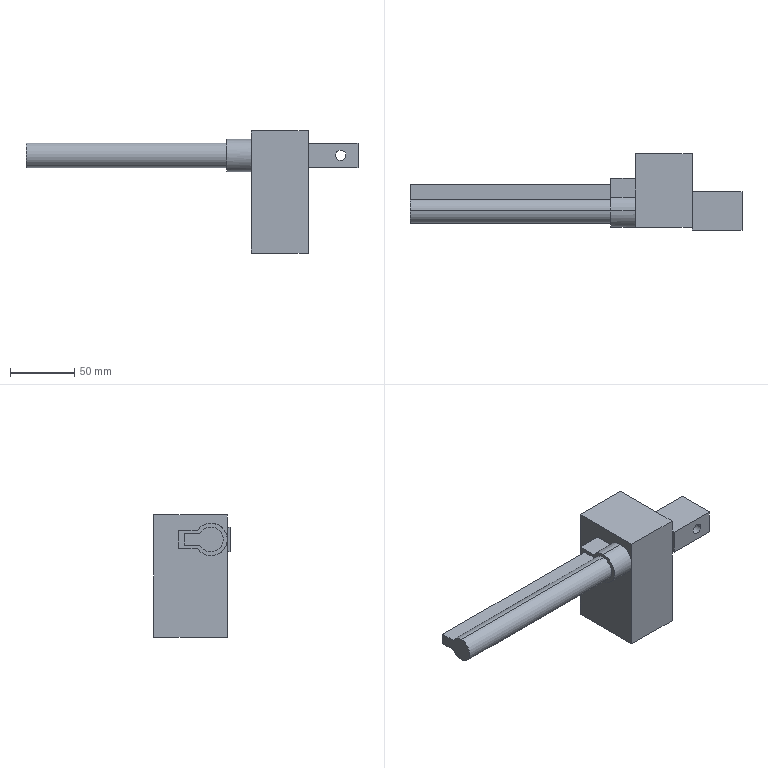Part | NX | features BREP 1 | 1 solid | 28 faces | box 259.112 x 59.436 x 95.25 mm | volume 337002 mm3 | plane 20 | cylinder 8 | commonest cylinder face diameters 19.304 x3 25.4 x3 8.255 x2
STEP:
#1=CARTESIAN_POINT('',(-19.05,25.4,6.985));
#2=VERTEX_POINT('',#1);
#3=CARTESIAN_POINT('',(-19.05,25.4,-6.985));
#4=VERTEX_POINT('',#3);
#5=CARTESIAN_POINT('',(-19.05,25.4,6.985));
#6=DIRECTION('',(0.,0.,-1.));
#7=VECTOR('',#6,1000.);
#8=LINE('',#5,#7);
#9=EDGE_CURVE('',#2,#4,#8,.T.);
#10=ORIENTED_EDGE('',*,*,#9,.T.);
#11=CARTESIAN_POINT('',(-19.05,10.607,-6.985));
#12=VERTEX_POINT('',#11);
#13=CARTESIAN_POINT('',(-19.05,25.4,-6.985));
#14=DIRECTION('',(0.,-1.,0.));
#15=VECTOR('',#14,1000.);
#16=LINE('',#13,#15);
#17=EDGE_CURVE('',#4,#12,#16,.T.);
#18=ORIENTED_EDGE('',*,*,#17,.T.);
#19=CARTESIAN_POINT('',(-19.05,0.,-12.7));
#20=VERTEX_POINT('',#19);
#21=CARTESIAN_POINT('',(-19.05,0.,0.));
#22=DIRECTION('',(-1.,0.,0.));
#23=DIRECTION('',(0.,0.8352,-0.55));
#24=AXIS2_PLACEMENT_3D('',#21,#22,#23);
#25=CIRCLE('',#24,12.7);
#26=EDGE_CURVE('',#12,#20,#25,.T.);
#27=ORIENTED_EDGE('',*,*,#26,.T.);
#28=CARTESIAN_POINT('',(-19.05,0.,12.7));
#29=VERTEX_POINT('',#28);
#30=CARTESIAN_POINT('',(-19.05,0.,0.));
#31=DIRECTION('',(-1.,0.,0.));
#32=DIRECTION('',(0.,0.8352,-0.55));
#33=AXIS2_PLACEMENT_3D('',#30,#31,#32);
#34=CIRCLE('',#33,12.7);
#35=EDGE_CURVE('',#20,#29,#34,.T.);
#36=ORIENTED_EDGE('',*,*,#35,.T.);
#37=CARTESIAN_POINT('',(-19.05,10.607,6.985));
#38=VERTEX_POINT('',#37);
#39=CARTESIAN_POINT('',(-19.05,0.,0.));
#40=DIRECTION('',(-1.,0.,0.));
#41=DIRECTION('',(0.,0.8352,-0.55));
#42=AXIS2_PLACEMENT_3D('',#39,#40,#41);
#43=CIRCLE('',#42,12.7);
#44=EDGE_CURVE('',#29,#38,#43,.T.);
#45=ORIENTED_EDGE('',*,*,#44,.T.);
#46=CARTESIAN_POINT('',(-19.05,10.607,6.985));
#47=DIRECTION('',(0.,1.,0.));
#48=VECTOR('',#47,1000.);
#49=LINE('',#46,#48);
#50=EDGE_CURVE('',#38,#2,#49,.T.);
#51=ORIENTED_EDGE('',*,*,#50,.T.);
#52=EDGE_LOOP('',(#10,#18,#27,#36,#45,#51));
#53=FACE_BOUND('',#52,.T.);
#54=CARTESIAN_POINT('',(-19.05,20.32,4.445));
#55=VERTEX_POINT('',#54);
#56=CARTESIAN_POINT('',(-19.05,20.32,-4.445));
#57=VERTEX_POINT('',#56);
#58=CARTESIAN_POINT('',(-19.05,20.32,4.445));
#59=DIRECTION('',(0.,0.,-1.));
#60=VECTOR('',#59,1000.);
#61=LINE('',#58,#60);
#62=EDGE_CURVE('',#55,#57,#61,.T.);
#63=ORIENTED_EDGE('',*,*,#62,.F.);
#64=CARTESIAN_POINT('',(-19.05,8.568,4.445));
#65=VERTEX_POINT('',#64);
#66=CARTESIAN_POINT('',(-19.05,8.568,4.445));
#67=DIRECTION('',(0.,1.,0.));
#68=VECTOR('',#67,1000.);
#69=LINE('',#66,#68);
#70=EDGE_CURVE('',#65,#55,#69,.T.);
#71=ORIENTED_EDGE('',*,*,#70,.F.);
#72=CARTESIAN_POINT('',(-19.05,0.,9.652));
#73=VERTEX_POINT('',#72);
#74=CARTESIAN_POINT('',(-19.05,0.,0.));
#75=DIRECTION('',(-1.,0.,0.));
#76=DIRECTION('',(0.,0.8876,-0.4605));
#77=AXIS2_PLACEMENT_3D('',#74,#75,#76);
#78=CIRCLE('',#77,9.652);
#79=EDGE_CURVE('',#73,#65,#78,.T.);
#80=ORIENTED_EDGE('',*,*,#79,.F.);
#81=CARTESIAN_POINT('',(-19.05,0.,-9.652));
#82=VERTEX_POINT('',#81);
#83=CARTESIAN_POINT('',(-19.05,0.,0.));
#84=DIRECTION('',(-1.,0.,0.));
#85=DIRECTION('',(0.,0.8876,-0.4605));
#86=AXIS2_PLACEMENT_3D('',#83,#84,#85);
#87=CIRCLE('',#86,9.652);
#88=EDGE_CURVE('',#82,#73,#87,.T.);
#89=ORIENTED_EDGE('',*,*,#88,.F.);
#90=CARTESIAN_POINT('',(-19.05,8.568,-4.445));
#91=VERTEX_POINT('',#90);
#92=CARTESIAN_POINT('',(-19.05,0.,0.));
#93=DIRECTION('',(-1.,0.,0.));
#94=DIRECTION('',(0.,0.8876,-0.4605));
#95=AXIS2_PLACEMENT_3D('',#92,#93,#94);
#96=CIRCLE('',#95,9.652);
#97=EDGE_CURVE('',#91,#82,#96,.T.);
#98=ORIENTED_EDGE('',*,*,#97,.F.);
#99=CARTESIAN_POINT('',(-19.05,20.32,-4.445));
#100=DIRECTION('',(0.,-1.,0.));
#101=VECTOR('',#100,1000.);
#102=LINE('',#99,#101);
#103=EDGE_CURVE('',#57,#91,#102,.T.);
#104=ORIENTED_EDGE('',*,*,#103,.F.);
#105=EDGE_LOOP('',(#63,#71,#80,#89,#98,#104));
#106=FACE_BOUND('',#105,.T.);
#107=CARTESIAN_POINT('',(-19.05,0.,0.));
#108=DIRECTION('',(1.,0.,0.));
#109=DIRECTION('',(0.,1.,0.));
#110=AXIS2_PLACEMENT_3D('',#107,#108,#109);
#111=PLANE('',#110);
#112=ADVANCED_FACE('',(#53,#106),#111,.F.);
#113=CARTESIAN_POINT('',(0.,25.4,6.985));
#114=VERTEX_POINT('',#113);
#115=CARTESIAN_POINT('',(-19.05,25.4,6.985));
#116=DIRECTION('',(1.,0.,0.));
#117=VECTOR('',#116,1000.);
#118=LINE('',#115,#117);
#119=EDGE_CURVE('',#2,#114,#118,.T.);
#120=ORIENTED_EDGE('',*,*,#119,.F.);
#121=ORIENTED_EDGE('',*,*,#50,.F.);
#122=CARTESIAN_POINT('',(0.,10.607,6.985));
#123=VERTEX_POINT('',#122);
#124=CARTESIAN_POINT('',(-19.05,10.607,6.985));
#125=DIRECTION('',(1.,0.,0.));
#126=VECTOR('',#125,1000.);
#127=LINE('',#124,#126);
#128=EDGE_CURVE('',#38,#123,#127,.T.);
#129=ORIENTED_EDGE('',*,*,#128,.T.);
#130=CARTESIAN_POINT('',(0.,25.4,6.985));
#131=DIRECTION('',(0.,-1.,0.));
#132=VECTOR('',#131,1000.);
#133=LINE('',#130,#132);
#134=EDGE_CURVE('',#114,#123,#133,.T.);
#135=ORIENTED_EDGE('',*,*,#134,.F.);
#136=EDGE_LOOP('',(#120,#121,#129,#135));
#137=FACE_BOUND('',#136,.T.);
#138=CARTESIAN_POINT('',(0.,25.4,6.985));
#139=DIRECTION('',(0.,0.,1.));
#140=DIRECTION('',(1.,0.,0.));
#141=AXIS2_PLACEMENT_3D('',#138,#139,#140);
#142=PLANE('',#141);
#143=ADVANCED_FACE('',(#137),#142,.T.);
#144=CARTESIAN_POINT('',(0.,0.,12.7));
#145=VERTEX_POINT('',#144);
#146=CARTESIAN_POINT('',(0.,0.,0.));
#147=DIRECTION('',(1.,0.,0.));
#148=DIRECTION('',(0.,0.8352,0.55));
#149=AXIS2_PLACEMENT_3D('',#146,#147,#148);
#150=CIRCLE('',#149,12.7);
#151=EDGE_CURVE('',#123,#145,#150,.T.);
#152=ORIENTED_EDGE('',*,*,#151,.T.);
#153=CARTESIAN_POINT('',(0.,-12.7,0.));
#154=VERTEX_POINT('',#153);
#155=CARTESIAN_POINT('',(0.,0.,0.));
#156=DIRECTION('',(1.,0.,0.));
#157=DIRECTION('',(0.,0.8352,0.55));
#158=AXIS2_PLACEMENT_3D('',#155,#156,#157);
#159=CIRCLE('',#158,12.7);
#160=EDGE_CURVE('',#145,#154,#159,.T.);
#161=ORIENTED_EDGE('',*,*,#160,.T.);
#162=CARTESIAN_POINT('',(0.,-12.7,19.05));
#163=VERTEX_POINT('',#162);
#164=CARTESIAN_POINT('',(0.,-12.7,0.));
#165=DIRECTION('',(0.,0.,1.));
#166=VECTOR('',#165,1000.);
#167=LINE('',#164,#166);
#168=EDGE_CURVE('',#154,#163,#167,.T.);
#169=ORIENTED_EDGE('',*,*,#168,.T.);
#170=CARTESIAN_POINT('',(0.,44.45,19.05));
#171=VERTEX_POINT('',#170);
#172=CARTESIAN_POINT('',(0.,44.45,19.05));
#173=DIRECTION('',(0.,-1.,0.));
#174=VECTOR('',#173,1000.);
#175=LINE('',#172,#174);
#176=EDGE_CURVE('',#171,#163,#175,.T.);
#177=ORIENTED_EDGE('',*,*,#176,.F.);
#178=CARTESIAN_POINT('',(0.,44.45,-76.2));
#179=VERTEX_POINT('',#178);
#180=CARTESIAN_POINT('',(0.,44.45,-76.2));
#181=DIRECTION('',(0.,0.,1.));
#182=VECTOR('',#181,1000.);
#183=LINE('',#180,#182);
#184=EDGE_CURVE('',#179,#171,#183,.T.);
#185=ORIENTED_EDGE('',*,*,#184,.F.);
#186=CARTESIAN_POINT('',(0.,-12.7,-76.2));
#187=VERTEX_POINT('',#186);
#188=CARTESIAN_POINT('',(0.,44.45,-76.2));
#189=DIRECTION('',(0.,-1.,0.));
#190=VECTOR('',#189,1000.);
#191=LINE('',#188,#190);
#192=EDGE_CURVE('',#179,#187,#191,.T.);
#193=ORIENTED_EDGE('',*,*,#192,.T.);
#194=CARTESIAN_POINT('',(0.,-12.7,-76.2));
#195=DIRECTION('',(0.,0.,1.));
#196=VECTOR('',#195,1000.);
#197=LINE('',#194,#196);
#198=EDGE_CURVE('',#187,#154,#197,.T.);
#199=ORIENTED_EDGE('',*,*,#198,.T.);
#200=CARTESIAN_POINT('',(0.,0.,-12.7));
#201=VERTEX_POINT('',#200);
#202=CARTESIAN_POINT('',(0.,0.,0.));
#203=DIRECTION('',(1.,0.,0.));
#204=DIRECTION('',(0.,-1.,0.));
#205=AXIS2_PLACEMENT_3D('',#202,#203,#204);
#206=CIRCLE('',#205,12.7);
#207=EDGE_CURVE('',#154,#201,#206,.T.);
#208=ORIENTED_EDGE('',*,*,#207,.T.);
#209=CARTESIAN_POINT('',(0.,10.607,-6.985));
#210=VERTEX_POINT('',#209);
#211=CARTESIAN_POINT('',(0.,0.,0.));
#212=DIRECTION('',(1.,0.,0.));
#213=DIRECTION('',(0.,-1.,0.));
#214=AXIS2_PLACEMENT_3D('',#211,#212,#213);
#215=CIRCLE('',#214,12.7);
#216=EDGE_CURVE('',#201,#210,#215,.T.);
#217=ORIENTED_EDGE('',*,*,#216,.T.);
#218=CARTESIAN_POINT('',(0.,25.4,-6.985));
#219=VERTEX_POINT('',#218);
#220=CARTESIAN_POINT('',(0.,10.607,-6.985));
#221=DIRECTION('',(0.,1.,0.));
#222=VECTOR('',#221,1000.);
#223=LINE('',#220,#222);
#224=EDGE_CURVE('',#210,#219,#223,.T.);
#225=ORIENTED_EDGE('',*,*,#224,.T.);
#226=CARTESIAN_POINT('',(0.,25.4,-6.985));
#227=DIRECTION('',(0.,0.,1.));
#228=VECTOR('',#227,1000.);
#229=LINE('',#226,#228);
#230=EDGE_CURVE('',#219,#114,#229,.T.);
#231=ORIENTED_EDGE('',*,*,#230,.T.);
#232=ORIENTED_EDGE('',*,*,#134,.T.);
#233=EDGE_LOOP('',(#152,#161,#169,#177,#185,#193,#199,#208,#217,#225,#231,#232));
#234=FACE_BOUND('',#233,.T.);
#235=CARTESIAN_POINT('',(0.,44.45,-76.2));
#236=DIRECTION('',(-1.,0.,0.));
#237=DIRECTION('',(0.,0.,1.));
#238=AXIS2_PLACEMENT_3D('',#235,#236,#237);
#239=PLANE('',#238);
#240=ADVANCED_FACE('',(#234),#239,.T.);
#241=CARTESIAN_POINT('',(-19.05,25.4,-6.985));
#242=DIRECTION('',(1.,0.,0.));
#243=VECTOR('',#242,1000.);
#244=LINE('',#241,#243);
#245=EDGE_CURVE('',#4,#219,#244,.T.);
#246=ORIENTED_EDGE('',*,*,#245,.F.);
#247=ORIENTED_EDGE('',*,*,#9,.F.);
#248=ORIENTED_EDGE('',*,*,#119,.T.);
#249=ORIENTED_EDGE('',*,*,#230,.F.);
#250=EDGE_LOOP('',(#246,#247,#248,#249));
#251=FACE_BOUND('',#250,.T.);
#252=CARTESIAN_POINT('',(0.,25.4,-6.985));
#253=DIRECTION('',(0.,1.,0.));
#254=DIRECTION('',(1.,0.,0.));
#255=AXIS2_PLACEMENT_3D('',#252,#253,#254);
#256=PLANE('',#255);
#257=ADVANCED_FACE('',(#251),#256,.T.);
#258=CARTESIAN_POINT('',(-19.05,10.607,-6.985));
#259=DIRECTION('',(1.,0.,0.));
#260=VECTOR('',#259,1000.);
#261=LINE('',#258,#260);
#262=EDGE_CURVE('',#12,#210,#261,.T.);
#263=ORIENTED_EDGE('',*,*,#262,.F.);
#264=ORIENTED_EDGE('',*,*,#17,.F.);
#265=ORIENTED_EDGE('',*,*,#245,.T.);
#266=ORIENTED_EDGE('',*,*,#224,.F.);
#267=EDGE_LOOP('',(#263,#264,#265,#266));
#268=FACE_BOUND('',#267,.T.);
#269=CARTESIAN_POINT('',(0.,10.607,-6.985));
#270=DIRECTION('',(0.,0.,-1.));
#271=DIRECTION('',(0.,-1.,0.));
#272=AXIS2_PLACEMENT_3D('',#269,#270,#271);
#273=PLANE('',#272);
#274=ADVANCED_FACE('',(#268),#273,.T.);
#275=CARTESIAN_POINT('',(0.,0.,-12.7));
#276=DIRECTION('',(1.,0.,0.));
#277=VECTOR('',#276,1000.);
#278=LINE('',#275,#277);
#279=EDGE_CURVE('',#20,#201,#278,.T.);
#280=ORIENTED_EDGE('',*,*,#279,.F.);
#281=ORIENTED_EDGE('',*,*,#26,.F.);
#282=ORIENTED_EDGE('',*,*,#262,.T.);
#283=ORIENTED_EDGE('',*,*,#216,.F.);
#284=EDGE_LOOP('',(#280,#281,#282,#283));
#285=FACE_BOUND('',#284,.T.);
#286=CARTESIAN_POINT('',(0.,0.,0.));
#287=DIRECTION('',(1.,0.,0.));
#288=DIRECTION('',(0.,0.,-1.));
#289=AXIS2_PLACEMENT_3D('',#286,#287,#288);
#290=CYLINDRICAL_SURFACE('',#289,12.7);
#291=ADVANCED_FACE('',(#285),#290,.T.);
#292=CARTESIAN_POINT('',(44.45,-12.7,9.525));
#293=VERTEX_POINT('',#292);
#294=CARTESIAN_POINT('',(44.45,-12.7,19.05));
#295=VERTEX_POINT('',#294);
#296=CARTESIAN_POINT('',(44.45,-12.7,9.525));
#297=DIRECTION('',(0.,0.,1.));
#298=VECTOR('',#297,1000.);
#299=LINE('',#296,#298);
#300=EDGE_CURVE('',#293,#295,#299,.T.);
#301=ORIENTED_EDGE('',*,*,#300,.T.);
#302=CARTESIAN_POINT('',(0.,-12.7,19.05));
#303=DIRECTION('',(1.,0.,0.));
#304=VECTOR('',#303,1000.);
#305=LINE('',#302,#304);
#306=EDGE_CURVE('',#163,#295,#305,.T.);
#307=ORIENTED_EDGE('',*,*,#306,.F.);
#308=ORIENTED_EDGE('',*,*,#168,.F.);
#309=ORIENTED_EDGE('',*,*,#198,.F.);
#310=CARTESIAN_POINT('',(44.45,-12.7,-76.2));
#311=VERTEX_POINT('',#310);
#312=CARTESIAN_POINT('',(0.,-12.7,-76.2));
#313=DIRECTION('',(1.,0.,0.));
#314=VECTOR('',#313,1000.);
#315=LINE('',#312,#314);
#316=EDGE_CURVE('',#187,#311,#315,.T.);
#317=ORIENTED_EDGE('',*,*,#316,.T.);
#318=CARTESIAN_POINT('',(44.45,-12.7,-9.525));
#319=VERTEX_POINT('',#318);
#320=CARTESIAN_POINT('',(44.45,-12.7,-76.2));
#321=DIRECTION('',(0.,0.,1.));
#322=VECTOR('',#321,1000.);
#323=LINE('',#320,#322);
#324=EDGE_CURVE('',#311,#319,#323,.T.);
#325=ORIENTED_EDGE('',*,*,#324,.T.);
#326=CARTESIAN_POINT('',(44.45,-12.7,-9.525));
#327=DIRECTION('',(0.,0.,1.));
#328=VECTOR('',#327,1000.);
#329=LINE('',#326,#328);
#330=EDGE_CURVE('',#319,#293,#329,.T.);
#331=ORIENTED_EDGE('',*,*,#330,.T.);
#332=EDGE_LOOP('',(#301,#307,#308,#309,#317,#325,#331));
#333=FACE_BOUND('',#332,.T.);
#334=CARTESIAN_POINT('',(0.,-12.7,-76.2));
#335=DIRECTION('',(0.,-1.,0.));
#336=DIRECTION('',(0.,0.,-1.));
#337=AXIS2_PLACEMENT_3D('',#334,#335,#336);
#338=PLANE('',#337);
#339=ADVANCED_FACE('',(#333),#338,.T.);
#340=CARTESIAN_POINT('',(44.45,-14.986,-9.525));
#341=VERTEX_POINT('',#340);
#342=CARTESIAN_POINT('',(44.45,-12.7,-9.525));
#343=DIRECTION('',(0.,-1.,0.));
#344=VECTOR('',#343,1000.);
#345=LINE('',#342,#344);
#346=EDGE_CURVE('',#319,#341,#345,.T.);
#347=ORIENTED_EDGE('',*,*,#346,.T.);
#348=CARTESIAN_POINT('',(44.45,-14.986,9.525));
#349=VERTEX_POINT('',#348);
#350=CARTESIAN_POINT('',(44.45,-14.986,-9.525));
#351=DIRECTION('',(0.,0.,1.));
#352=VECTOR('',#351,1000.);
#353=LINE('',#350,#352);
#354=EDGE_CURVE('',#341,#349,#353,.T.);
#355=ORIENTED_EDGE('',*,*,#354,.T.);
#356=CARTESIAN_POINT('',(44.45,-12.7,9.525));
#357=DIRECTION('',(0.,-1.,0.));
#358=VECTOR('',#357,1000.);
#359=LINE('',#356,#358);
#360=EDGE_CURVE('',#293,#349,#359,.T.);
#361=ORIENTED_EDGE('',*,*,#360,.F.);
#362=ORIENTED_EDGE('',*,*,#330,.F.);
#363=EDGE_LOOP('',(#347,#355,#361,#362));
#364=FACE_BOUND('',#363,.T.);
#365=CARTESIAN_POINT('',(44.45,14.986,-9.525));
#366=DIRECTION('',(-1.,0.,0.));
#367=DIRECTION('',(0.,0.,1.));
#368=AXIS2_PLACEMENT_3D('',#365,#366,#367);
#369=PLANE('',#368);
#370=ADVANCED_FACE('',(#364),#369,.T.);
#371=ORIENTED_EDGE('',*,*,#360,.T.);
#372=CARTESIAN_POINT('',(83.344,-14.986,9.525));
#373=VERTEX_POINT('',#372);
#374=CARTESIAN_POINT('',(44.45,-14.986,9.525));
#375=DIRECTION('',(1.,0.,0.));
#376=VECTOR('',#375,1000.);
#377=LINE('',#374,#376);
#378=EDGE_CURVE('',#349,#373,#377,.T.);
#379=ORIENTED_EDGE('',*,*,#378,.T.);
#380=CARTESIAN_POINT('',(83.344,14.986,9.525));
#381=VERTEX_POINT('',#380);
#382=CARTESIAN_POINT('',(83.344,-14.986,9.525));
#383=DIRECTION('',(0.,1.,0.));
#384=VECTOR('',#383,1000.);
#385=LINE('',#382,#384);
#386=EDGE_CURVE('',#373,#381,#385,.T.);
#387=ORIENTED_EDGE('',*,*,#386,.T.);
#388=CARTESIAN_POINT('',(44.45,14.986,9.525));
#389=VERTEX_POINT('',#388);
#390=CARTESIAN_POINT('',(83.344,14.986,9.525));
#391=DIRECTION('',(-1.,0.,0.));
#392=VECTOR('',#391,1000.);
#393=LINE('',#390,#392);
#394=EDGE_CURVE('',#381,#389,#393,.T.);
#395=ORIENTED_EDGE('',*,*,#394,.T.);
#396=CARTESIAN_POINT('',(44.45,-12.7,9.525));
#397=DIRECTION('',(0.,1.,0.));
#398=VECTOR('',#397,1000.);
#399=LINE('',#396,#398);
#400=EDGE_CURVE('',#293,#389,#399,.T.);
#401=ORIENTED_EDGE('',*,*,#400,.F.);
#402=EDGE_LOOP('',(#371,#379,#387,#395,#401));
#403=FACE_BOUND('',#402,.T.);
#404=CARTESIAN_POINT('',(0.,0.,9.525));
#405=DIRECTION('',(0.,0.,1.));
#406=DIRECTION('',(1.,0.,0.));
#407=AXIS2_PLACEMENT_3D('',#404,#405,#406);
#408=PLANE('',#407);
#409=ADVANCED_FACE('',(#403),#408,.T.);
#410=ORIENTED_EDGE('',*,*,#324,.F.);
#411=CARTESIAN_POINT('',(44.45,44.45,-76.2));
#412=VERTEX_POINT('',#411);
#413=CARTESIAN_POINT('',(44.45,-12.7,-76.2));
#414=DIRECTION('',(0.,1.,0.));
#415=VECTOR('',#414,1000.);
#416=LINE('',#413,#415);
#417=EDGE_CURVE('',#311,#412,#416,.T.);
#418=ORIENTED_EDGE('',*,*,#417,.T.);
#419=CARTESIAN_POINT('',(44.45,44.45,19.05));
#420=VERTEX_POINT('',#419);
#421=CARTESIAN_POINT('',(44.45,44.45,-76.2));
#422=DIRECTION('',(0.,0.,1.));
#423=VECTOR('',#422,1000.);
#424=LINE('',#421,#423);
#425=EDGE_CURVE('',#412,#420,#424,.T.);
#426=ORIENTED_EDGE('',*,*,#425,.T.);
#427=CARTESIAN_POINT('',(44.45,-12.7,19.05));
#428=DIRECTION('',(0.,1.,0.));
#429=VECTOR('',#428,1000.);
#430=LINE('',#427,#429);
#431=EDGE_CURVE('',#295,#420,#430,.T.);
#432=ORIENTED_EDGE('',*,*,#431,.F.);
#433=ORIENTED_EDGE('',*,*,#300,.F.);
#434=ORIENTED_EDGE('',*,*,#400,.T.);
#435=CARTESIAN_POINT('',(44.45,14.986,-9.525));
#436=VERTEX_POINT('',#435);
#437=CARTESIAN_POINT('',(44.45,14.986,-9.525));
#438=DIRECTION('',(0.,0.,1.));
#439=VECTOR('',#438,1000.);
#440=LINE('',#437,#439);
#441=EDGE_CURVE('',#436,#389,#440,.T.);
#442=ORIENTED_EDGE('',*,*,#441,.F.);
#443=CARTESIAN_POINT('',(44.45,-12.7,-9.525));
#444=DIRECTION('',(0.,1.,0.));
#445=VECTOR('',#444,1000.);
#446=LINE('',#443,#445);
#447=EDGE_CURVE('',#319,#436,#446,.T.);
#448=ORIENTED_EDGE('',*,*,#447,.F.);
#449=EDGE_LOOP('',(#410,#418,#426,#432,#433,#434,#442,#448));
#450=FACE_BOUND('',#449,.T.);
#451=CARTESIAN_POINT('',(44.45,-12.7,-76.2));
#452=DIRECTION('',(1.,0.,0.));
#453=DIRECTION('',(0.,1.,0.));
#454=AXIS2_PLACEMENT_3D('',#451,#452,#453);
#455=PLANE('',#454);
#456=ADVANCED_FACE('',(#450),#455,.T.);
#457=CARTESIAN_POINT('',(83.344,14.986,-9.525));
#458=VERTEX_POINT('',#457);
#459=CARTESIAN_POINT('',(83.344,14.986,-9.525));
#460=DIRECTION('',(-1.,0.,0.));
#461=VECTOR('',#460,1000.);
#462=LINE('',#459,#461);
#463=EDGE_CURVE('',#458,#436,#462,.T.);
#464=ORIENTED_EDGE('',*,*,#463,.F.);
#465=CARTESIAN_POINT('',(83.344,-14.986,-9.525));
#466=VERTEX_POINT('',#465);
#467=CARTESIAN_POINT('',(83.344,-14.986,-9.525));
#468=DIRECTION('',(0.,1.,0.));
#469=VECTOR('',#468,1000.);
#470=LINE('',#467,#469);
#471=EDGE_CURVE('',#466,#458,#470,.T.);
#472=ORIENTED_EDGE('',*,*,#471,.F.);
#473=CARTESIAN_POINT('',(44.45,-14.986,-9.525));
#474=DIRECTION('',(1.,0.,0.));
#475=VECTOR('',#474,1000.);
#476=LINE('',#473,#475);
#477=EDGE_CURVE('',#341,#466,#476,.T.);
#478=ORIENTED_EDGE('',*,*,#477,.F.);
#479=ORIENTED_EDGE('',*,*,#346,.F.);
#480=ORIENTED_EDGE('',*,*,#447,.T.);
#481=EDGE_LOOP('',(#464,#472,#478,#479,#480));
#482=FACE_BOUND('',#481,.T.);
#483=CARTESIAN_POINT('',(0.,0.,-9.525));
#484=DIRECTION('',(0.,0.,1.));
#485=DIRECTION('',(1.,0.,0.));
#486=AXIS2_PLACEMENT_3D('',#483,#484,#485);
#487=PLANE('',#486);
#488=ADVANCED_FACE('',(#482),#487,.F.);
#489=CARTESIAN_POINT('',(83.344,-14.986,-9.525));
#490=DIRECTION('',(0.,0.,1.));
#491=VECTOR('',#490,1000.);
#492=LINE('',#489,#491);
#493=EDGE_CURVE('',#466,#373,#492,.T.);
#494=ORIENTED_EDGE('',*,*,#493,.T.);
#495=ORIENTED_EDGE('',*,*,#378,.F.);
#496=ORIENTED_EDGE('',*,*,#354,.F.);
#497=ORIENTED_EDGE('',*,*,#477,.T.);
#498=EDGE_LOOP('',(#494,#495,#496,#497));
#499=FACE_BOUND('',#498,.T.);
#500=CARTESIAN_POINT('',(65.722,-14.986,0.));
#501=VERTEX_POINT('',#500);
#502=CARTESIAN_POINT('',(73.978,-14.986,0.));
#503=VERTEX_POINT('',#502);
#504=CARTESIAN_POINT('',(69.85,-14.986,0.));
#505=DIRECTION('',(0.,-1.,0.));
#506=DIRECTION('',(-1.,0.,0.));
#507=AXIS2_PLACEMENT_3D('',#504,#505,#506);
#508=CIRCLE('',#507,4.128);
#509=EDGE_CURVE('',#501,#503,#508,.T.);
#510=ORIENTED_EDGE('',*,*,#509,.F.);
#511=CARTESIAN_POINT('',(69.85,-14.986,0.));
#512=DIRECTION('',(0.,-1.,0.));
#513=DIRECTION('',(1.,0.,0.));
#514=AXIS2_PLACEMENT_3D('',#511,#512,#513);
#515=CIRCLE('',#514,4.128);
#516=EDGE_CURVE('',#503,#501,#515,.T.);
#517=ORIENTED_EDGE('',*,*,#516,.F.);
#518=EDGE_LOOP('',(#510,#517));
#519=FACE_BOUND('',#518,.T.);
#520=CARTESIAN_POINT('',(44.45,-14.986,-9.525));
#521=DIRECTION('',(0.,-1.,0.));
#522=DIRECTION('',(0.,0.,-1.));
#523=AXIS2_PLACEMENT_3D('',#520,#521,#522);
#524=PLANE('',#523);
#525=ADVANCED_FACE('',(#499,#519),#524,.T.);
#526=CARTESIAN_POINT('',(83.344,14.986,-9.525));
#527=DIRECTION('',(0.,0.,1.));
#528=VECTOR('',#527,1000.);
#529=LINE('',#526,#528);
#530=EDGE_CURVE('',#458,#381,#529,.T.);
#531=ORIENTED_EDGE('',*,*,#530,.T.);
#532=ORIENTED_EDGE('',*,*,#386,.F.);
#533=ORIENTED_EDGE('',*,*,#493,.F.);
#534=ORIENTED_EDGE('',*,*,#471,.T.);
#535=EDGE_LOOP('',(#531,#532,#533,#534));
#536=FACE_BOUND('',#535,.T.);
#537=CARTESIAN_POINT('',(83.344,-14.986,-9.525));
#538=DIRECTION('',(1.,0.,0.));
#539=DIRECTION('',(0.,1.,0.));
#540=AXIS2_PLACEMENT_3D('',#537,#538,#539);
#541=PLANE('',#540);
#542=ADVANCED_FACE('',(#536),#541,.T.);
#543=ORIENTED_EDGE('',*,*,#394,.F.);
#544=ORIENTED_EDGE('',*,*,#530,.F.);
#545=ORIENTED_EDGE('',*,*,#463,.T.);
#546=ORIENTED_EDGE('',*,*,#441,.T.);
#547=EDGE_LOOP('',(#543,#544,#545,#546));
#548=FACE_BOUND('',#547,.T.);
#549=CARTESIAN_POINT('',(65.722,14.986,0.));
#550=VERTEX_POINT('',#549);
#551=CARTESIAN_POINT('',(73.978,14.986,0.));
#552=VERTEX_POINT('',#551);
#553=CARTESIAN_POINT('',(69.85,14.986,0.));
#554=DIRECTION('',(0.,-1.,0.));
#555=DIRECTION('',(-1.,0.,0.));
#556=AXIS2_PLACEMENT_3D('',#553,#554,#555);
#557=CIRCLE('',#556,4.128);
#558=EDGE_CURVE('',#550,#552,#557,.T.);
#559=ORIENTED_EDGE('',*,*,#558,.T.);
#560=CARTESIAN_POINT('',(69.85,14.986,0.));
#561=DIRECTION('',(0.,-1.,0.));
#562=DIRECTION('',(1.,0.,0.));
#563=AXIS2_PLACEMENT_3D('',#560,#561,#562);
#564=CIRCLE('',#563,4.128);
#565=EDGE_CURVE('',#552,#550,#564,.T.);
#566=ORIENTED_EDGE('',*,*,#565,.T.);
#567=EDGE_LOOP('',(#559,#566));
#568=FACE_BOUND('',#567,.T.);
#569=CARTESIAN_POINT('',(83.344,14.986,-9.525));
#570=DIRECTION('',(0.,1.,0.));
#571=DIRECTION('',(1.,0.,0.));
#572=AXIS2_PLACEMENT_3D('',#569,#570,#571);
#573=PLANE('',#572);
#574=ADVANCED_FACE('',(#548,#568),#573,.T.);
#575=ORIENTED_EDGE('',*,*,#516,.T.);
#576=CARTESIAN_POINT('',(65.722,14.986,0.));
#577=DIRECTION('',(0.,-1.,0.));
#578=VECTOR('',#577,1000.);
#579=LINE('',#576,#578);
#580=EDGE_CURVE('',#501,#550,#579,.F.);
#581=ORIENTED_EDGE('',*,*,#580,.T.);
#582=ORIENTED_EDGE('',*,*,#565,.F.);
#583=CARTESIAN_POINT('',(73.978,14.986,0.));
#584=DIRECTION('',(0.,-1.,0.));
#585=VECTOR('',#584,1000.);
#586=LINE('',#583,#585);
#587=EDGE_CURVE('',#503,#552,#586,.F.);
#588=ORIENTED_EDGE('',*,*,#587,.F.);
#589=EDGE_LOOP('',(#575,#581,#582,#588));
#590=FACE_BOUND('',#589,.T.);
#591=CARTESIAN_POINT('',(69.85,14.986,0.));
#592=DIRECTION('',(0.,-1.,0.));
#593=DIRECTION('',(1.,0.,0.));
#594=AXIS2_PLACEMENT_3D('',#591,#592,#593);
#595=CYLINDRICAL_SURFACE('',#594,4.128);
#596=ADVANCED_FACE('',(#590),#595,.F.);
#597=ORIENTED_EDGE('',*,*,#558,.F.);
#598=ORIENTED_EDGE('',*,*,#580,.F.);
#599=ORIENTED_EDGE('',*,*,#509,.T.);
#600=ORIENTED_EDGE('',*,*,#587,.T.);
#601=EDGE_LOOP('',(#597,#598,#599,#600));
#602=FACE_BOUND('',#601,.T.);
#603=CARTESIAN_POINT('',(69.85,14.986,0.));
#604=DIRECTION('',(0.,-1.,0.));
#605=DIRECTION('',(1.,0.,0.));
#606=AXIS2_PLACEMENT_3D('',#603,#604,#605);
#607=CYLINDRICAL_SURFACE('',#606,4.128);
#608=ADVANCED_FACE('',(#602),#607,.F.);
#609=ORIENTED_EDGE('',*,*,#306,.T.);
#610=ORIENTED_EDGE('',*,*,#431,.T.);
#611=CARTESIAN_POINT('',(44.45,44.45,19.05));
#612=DIRECTION('',(-1.,0.,0.));
#613=VECTOR('',#612,1000.);
#614=LINE('',#611,#613);
#615=EDGE_CURVE('',#420,#171,#614,.T.);
#616=ORIENTED_EDGE('',*,*,#615,.T.);
#617=ORIENTED_EDGE('',*,*,#176,.T.);
#618=EDGE_LOOP('',(#609,#610,#616,#617));
#619=FACE_BOUND('',#618,.T.);
#620=CARTESIAN_POINT('',(0.,0.,19.05));
#621=DIRECTION('',(0.,0.,1.));
#622=DIRECTION('',(1.,0.,0.));
#623=AXIS2_PLACEMENT_3D('',#620,#621,#622);
#624=PLANE('',#623);
#625=ADVANCED_FACE('',(#619),#624,.T.);
#626=ORIENTED_EDGE('',*,*,#184,.T.);
#627=ORIENTED_EDGE('',*,*,#615,.F.);
#628=ORIENTED_EDGE('',*,*,#425,.F.);
#629=CARTESIAN_POINT('',(44.45,44.45,-76.2));
#630=DIRECTION('',(-1.,0.,0.));
#631=VECTOR('',#630,1000.);
#632=LINE('',#629,#631);
#633=EDGE_CURVE('',#412,#179,#632,.T.);
#634=ORIENTED_EDGE('',*,*,#633,.T.);
#635=EDGE_LOOP('',(#626,#627,#628,#634));
#636=FACE_BOUND('',#635,.T.);
#637=CARTESIAN_POINT('',(44.45,44.45,-76.2));
#638=DIRECTION('',(0.,1.,0.));
#639=DIRECTION('',(1.,0.,0.));
#640=AXIS2_PLACEMENT_3D('',#637,#638,#639);
#641=PLANE('',#640);
#642=ADVANCED_FACE('',(#636),#641,.T.);
#643=ORIENTED_EDGE('',*,*,#633,.F.);
#644=ORIENTED_EDGE('',*,*,#417,.F.);
#645=ORIENTED_EDGE('',*,*,#316,.F.);
#646=ORIENTED_EDGE('',*,*,#192,.F.);
#647=EDGE_LOOP('',(#643,#644,#645,#646));
#648=FACE_BOUND('',#647,.T.);
#649=CARTESIAN_POINT('',(0.,0.,-76.2));
#650=DIRECTION('',(0.,0.,1.));
#651=DIRECTION('',(1.,0.,0.));
#652=AXIS2_PLACEMENT_3D('',#649,#650,#651);
#653=PLANE('',#652);
#654=ADVANCED_FACE('',(#648),#653,.F.);
#655=CARTESIAN_POINT('',(-175.768,8.568,-4.445));
#656=VERTEX_POINT('',#655);
#657=CARTESIAN_POINT('',(-19.05,8.568,-4.445));
#658=DIRECTION('',(-1.,0.,0.));
#659=VECTOR('',#658,1000.);
#660=LINE('',#657,#659);
#661=EDGE_CURVE('',#91,#656,#660,.T.);
#662=ORIENTED_EDGE('',*,*,#661,.T.);
#663=CARTESIAN_POINT('',(-175.768,20.32,-4.445));
#664=VERTEX_POINT('',#663);
#665=CARTESIAN_POINT('',(-175.768,20.32,-4.445));
#666=DIRECTION('',(0.,-1.,0.));
#667=VECTOR('',#666,1000.);
#668=LINE('',#665,#667);
#669=EDGE_CURVE('',#664,#656,#668,.T.);
#670=ORIENTED_EDGE('',*,*,#669,.F.);
#671=CARTESIAN_POINT('',(-19.05,20.32,-4.445));
#672=DIRECTION('',(-1.,0.,0.));
#673=VECTOR('',#672,1000.);
#674=LINE('',#671,#673);
#675=EDGE_CURVE('',#57,#664,#674,.T.);
#676=ORIENTED_EDGE('',*,*,#675,.F.);
#677=ORIENTED_EDGE('',*,*,#103,.T.);
#678=EDGE_LOOP('',(#662,#670,#676,#677));
#679=FACE_BOUND('',#678,.T.);
#680=CARTESIAN_POINT('',(-19.05,20.32,-4.445));
#681=DIRECTION('',(0.,0.,-1.));
#682=DIRECTION('',(0.,-1.,0.));
#683=AXIS2_PLACEMENT_3D('',#680,#681,#682);
#684=PLANE('',#683);
#685=ADVANCED_FACE('',(#679),#684,.T.);
#686=ORIENTED_EDGE('',*,*,#675,.T.);
#687=CARTESIAN_POINT('',(-175.768,20.32,4.445));
#688=VERTEX_POINT('',#687);
#689=CARTESIAN_POINT('',(-175.768,20.32,4.445));
#690=DIRECTION('',(0.,0.,-1.));
#691=VECTOR('',#690,1000.);
#692=LINE('',#689,#691);
#693=EDGE_CURVE('',#688,#664,#692,.T.);
#694=ORIENTED_EDGE('',*,*,#693,.F.);
#695=CARTESIAN_POINT('',(-19.05,20.32,4.445));
#696=DIRECTION('',(-1.,0.,0.));
#697=VECTOR('',#696,1000.);
#698=LINE('',#695,#697);
#699=EDGE_CURVE('',#55,#688,#698,.T.);
#700=ORIENTED_EDGE('',*,*,#699,.F.);
#701=ORIENTED_EDGE('',*,*,#62,.T.);
#702=EDGE_LOOP('',(#686,#694,#700,#701));
#703=FACE_BOUND('',#702,.T.);
#704=CARTESIAN_POINT('',(-19.05,20.32,4.445));
#705=DIRECTION('',(0.,1.,0.));
#706=DIRECTION('',(1.,0.,0.));
#707=AXIS2_PLACEMENT_3D('',#704,#705,#706);
#708=PLANE('',#707);
#709=ADVANCED_FACE('',(#703),#708,.T.);
#710=ORIENTED_EDGE('',*,*,#699,.T.);
#711=CARTESIAN_POINT('',(-175.768,8.568,4.445));
#712=VERTEX_POINT('',#711);
#713=CARTESIAN_POINT('',(-175.768,8.568,4.445));
#714=DIRECTION('',(0.,1.,0.));
#715=VECTOR('',#714,1000.);
#716=LINE('',#713,#715);
#717=EDGE_CURVE('',#712,#688,#716,.T.);
#718=ORIENTED_EDGE('',*,*,#717,.F.);
#719=CARTESIAN_POINT('',(-19.05,8.568,4.445));
#720=DIRECTION('',(-1.,0.,0.));
#721=VECTOR('',#720,1000.);
#722=LINE('',#719,#721);
#723=EDGE_CURVE('',#65,#712,#722,.T.);
#724=ORIENTED_EDGE('',*,*,#723,.F.);
#725=ORIENTED_EDGE('',*,*,#70,.T.);
#726=EDGE_LOOP('',(#710,#718,#724,#725));
#727=FACE_BOUND('',#726,.T.);
#728=CARTESIAN_POINT('',(-19.05,8.568,4.445));
#729=DIRECTION('',(0.,0.,1.));
#730=DIRECTION('',(1.,0.,0.));
#731=AXIS2_PLACEMENT_3D('',#728,#729,#730);
#732=PLANE('',#731);
#733=ADVANCED_FACE('',(#727),#732,.T.);
#734=CARTESIAN_POINT('',(-175.768,0.,9.652));
#735=VERTEX_POINT('',#734);
#736=CARTESIAN_POINT('',(-19.05,0.,9.652));
#737=DIRECTION('',(-1.,0.,0.));
#738=VECTOR('',#737,1000.);
#739=LINE('',#736,#738);
#740=EDGE_CURVE('',#73,#735,#739,.T.);
#741=ORIENTED_EDGE('',*,*,#740,.F.);
#742=ORIENTED_EDGE('',*,*,#79,.T.);
#743=ORIENTED_EDGE('',*,*,#723,.T.);
#744=CARTESIAN_POINT('',(-175.768,0.,0.));
#745=DIRECTION('',(-1.,0.,0.));
#746=DIRECTION('',(0.,0.8876,-0.4605));
#747=AXIS2_PLACEMENT_3D('',#744,#745,#746);
#748=CIRCLE('',#747,9.652);
#749=EDGE_CURVE('',#735,#712,#748,.T.);
#750=ORIENTED_EDGE('',*,*,#749,.F.);
#751=EDGE_LOOP('',(#741,#742,#743,#750));
#752=FACE_BOUND('',#751,.T.);
#753=CARTESIAN_POINT('',(-19.05,0.,0.));
#754=DIRECTION('',(-1.,0.,0.));
#755=DIRECTION('',(0.,0.,1.));
#756=AXIS2_PLACEMENT_3D('',#753,#754,#755);
#757=CYLINDRICAL_SURFACE('',#756,9.652);
#758=ADVANCED_FACE('',(#752),#757,.T.);
#759=CARTESIAN_POINT('',(-175.768,0.,-9.652));
#760=VERTEX_POINT('',#759);
#761=CARTESIAN_POINT('',(-175.768,0.,0.));
#762=DIRECTION('',(-1.,0.,0.));
#763=DIRECTION('',(0.,0.8876,-0.4605));
#764=AXIS2_PLACEMENT_3D('',#761,#762,#763);
#765=CIRCLE('',#764,9.652);
#766=EDGE_CURVE('',#656,#760,#765,.T.);
#767=ORIENTED_EDGE('',*,*,#766,.T.);
#768=CARTESIAN_POINT('',(-175.768,0.,0.));
#769=DIRECTION('',(-1.,0.,0.));
#770=DIRECTION('',(0.,0.8876,-0.4605));
#771=AXIS2_PLACEMENT_3D('',#768,#769,#770);
#772=CIRCLE('',#771,9.652);
#773=EDGE_CURVE('',#760,#735,#772,.T.);
#774=ORIENTED_EDGE('',*,*,#773,.T.);
#775=ORIENTED_EDGE('',*,*,#749,.T.);
#776=ORIENTED_EDGE('',*,*,#717,.T.);
#777=ORIENTED_EDGE('',*,*,#693,.T.);
#778=ORIENTED_EDGE('',*,*,#669,.T.);
#779=EDGE_LOOP('',(#767,#774,#775,#776,#777,#778));
#780=FACE_BOUND('',#779,.T.);
#781=CARTESIAN_POINT('',(-175.768,14.986,0.));
#782=DIRECTION('',(1.,0.,0.));
#783=DIRECTION('',(0.,1.,0.));
#784=AXIS2_PLACEMENT_3D('',#781,#782,#783);
#785=PLANE('',#784);
#786=ADVANCED_FACE('',(#780),#785,.F.);
#787=CARTESIAN_POINT('',(-19.05,0.,-9.652));
#788=DIRECTION('',(-1.,0.,0.));
#789=VECTOR('',#788,1000.);
#790=LINE('',#787,#789);
#791=EDGE_CURVE('',#82,#760,#790,.T.);
#792=ORIENTED_EDGE('',*,*,#791,.F.);
#793=ORIENTED_EDGE('',*,*,#88,.T.);
#794=ORIENTED_EDGE('',*,*,#740,.T.);
#795=ORIENTED_EDGE('',*,*,#773,.F.);
#796=EDGE_LOOP('',(#792,#793,#794,#795));
#797=FACE_BOUND('',#796,.T.);
#798=CARTESIAN_POINT('',(-19.05,0.,0.));
#799=DIRECTION('',(-1.,0.,0.));
#800=DIRECTION('',(0.,0.,1.));
#801=AXIS2_PLACEMENT_3D('',#798,#799,#800);
#802=CYLINDRICAL_SURFACE('',#801,9.652);
#803=ADVANCED_FACE('',(#797),#802,.T.);
#804=ORIENTED_EDGE('',*,*,#97,.T.);
#805=ORIENTED_EDGE('',*,*,#791,.T.);
#806=ORIENTED_EDGE('',*,*,#766,.F.);
#807=ORIENTED_EDGE('',*,*,#661,.F.);
#808=EDGE_LOOP('',(#804,#805,#806,#807));
#809=FACE_BOUND('',#808,.T.);
#810=CARTESIAN_POINT('',(-19.05,0.,0.));
#811=DIRECTION('',(-1.,0.,0.));
#812=DIRECTION('',(0.,0.,1.));
#813=AXIS2_PLACEMENT_3D('',#810,#811,#812);
#814=CYLINDRICAL_SURFACE('',#813,9.652);
#815=ADVANCED_FACE('',(#809),#814,.T.);
#816=CARTESIAN_POINT('',(0.,0.,12.7));
#817=DIRECTION('',(1.,0.,0.));
#818=VECTOR('',#817,1000.);
#819=LINE('',#816,#818);
#820=EDGE_CURVE('',#29,#145,#819,.T.);
#821=ORIENTED_EDGE('',*,*,#820,.F.);
#822=ORIENTED_EDGE('',*,*,#35,.F.);
#823=ORIENTED_EDGE('',*,*,#279,.T.);
#824=ORIENTED_EDGE('',*,*,#207,.F.);
#825=ORIENTED_EDGE('',*,*,#160,.F.);
#826=EDGE_LOOP('',(#821,#822,#823,#824,#825));
#827=FACE_BOUND('',#826,.T.);
#828=CARTESIAN_POINT('',(0.,0.,0.));
#829=DIRECTION('',(1.,0.,0.));
#830=DIRECTION('',(0.,0.,-1.));
#831=AXIS2_PLACEMENT_3D('',#828,#829,#830);
#832=CYLINDRICAL_SURFACE('',#831,12.7);
#833=ADVANCED_FACE('',(#827),#832,.T.);
#834=ORIENTED_EDGE('',*,*,#44,.F.);
#835=ORIENTED_EDGE('',*,*,#820,.T.);
#836=ORIENTED_EDGE('',*,*,#151,.F.);
#837=ORIENTED_EDGE('',*,*,#128,.F.);
#838=EDGE_LOOP('',(#834,#835,#836,#837));
#839=FACE_BOUND('',#838,.T.);
#840=CARTESIAN_POINT('',(0.,0.,0.));
#841=DIRECTION('',(1.,0.,0.));
#842=DIRECTION('',(0.,0.,-1.));
#843=AXIS2_PLACEMENT_3D('',#840,#841,#842);
#844=CYLINDRICAL_SURFACE('',#843,12.7);
#845=ADVANCED_FACE('',(#839),#844,.T.);
#846=CLOSED_SHELL('',(#112,#143,#240,#257,#274,#291,#339,#370,#409,#456,#488,#525,#542,#574,#596,#608,#625,#642,#654,#685,#709,#733,#758,#786,#803,#815,#833,#845));
#847=MANIFOLD_SOLID_BREP('',#846);
#848=(LENGTH_UNIT()NAMED_UNIT(*)SI_UNIT(.MILLI.,.METRE.));
#849=UNCERTAINTY_MEASURE_WITH_UNIT(LENGTH_MEASURE(0.00001),#848,'','');
#850=(NAMED_UNIT(*)PLANE_ANGLE_UNIT()SI_UNIT($,.RADIAN.));
#851=(NAMED_UNIT(*)SI_UNIT($,.STERADIAN.)SOLID_ANGLE_UNIT());
#852=(GEOMETRIC_REPRESENTATION_CONTEXT(3)GLOBAL_UNCERTAINTY_ASSIGNED_CONTEXT((#849))GLOBAL_UNIT_ASSIGNED_CONTEXT((#848,#850,#851))REPRESENTATION_CONTEXT('',''));
#853=ADVANCED_BREP_SHAPE_REPRESENTATION('',(#847),#852);